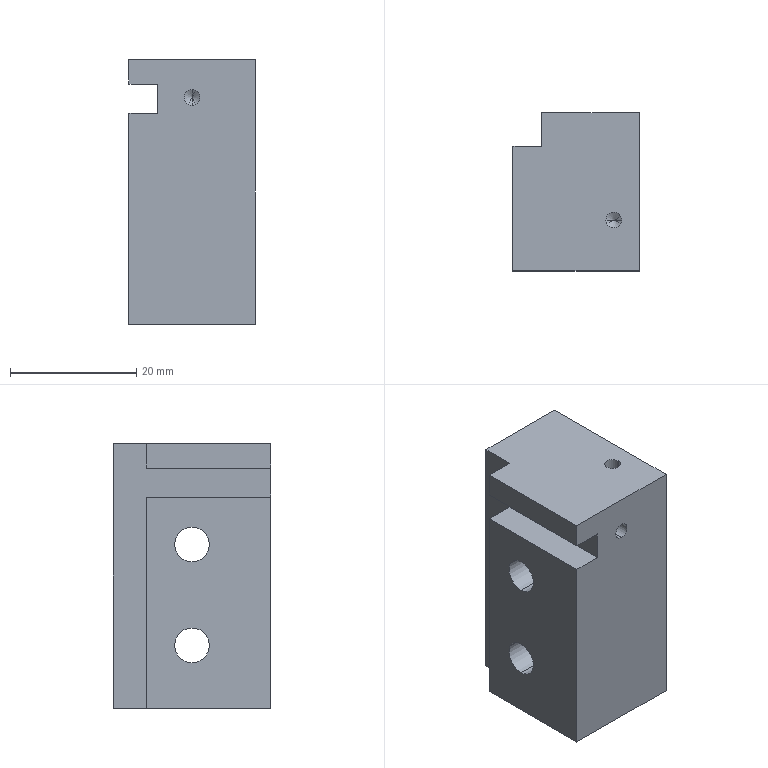Part | STEP file | Rivet press-in harpoon track_Default | 1 solid | 30 faces | box 20 x 25 x 42 mm | volume 18009 mm3 | plane 14 | cylinder 12 | cone 4 | commonest cylinder face diameters 2.5 x4 5.5 x4 9.5 x4